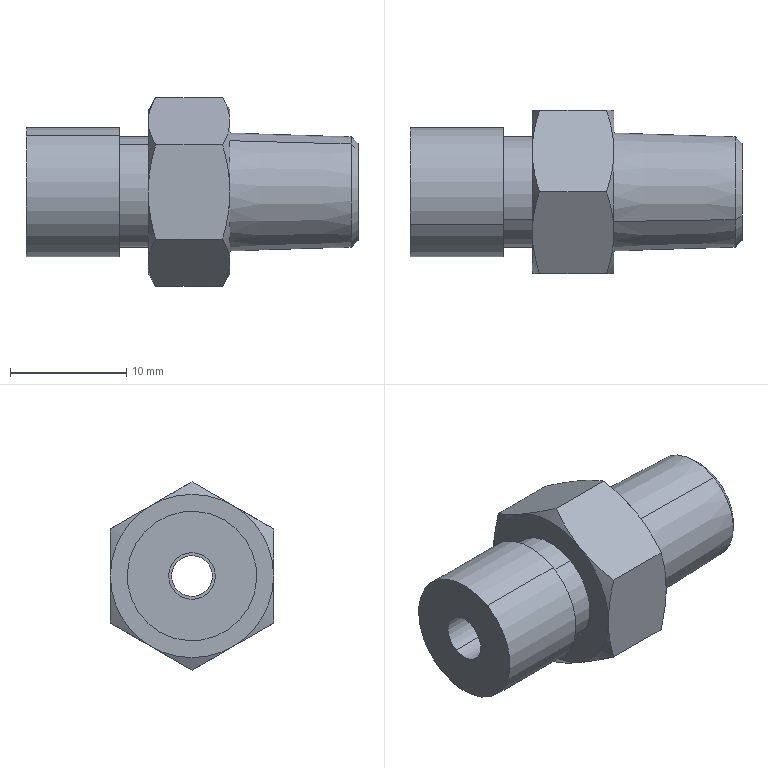Part | STEP file | SKTGK4-1-Part-1-1 | 1 solid | 36 faces | box 28.5 x 14 x 16.166 mm | volume 2666 mm3 | cone 16 | plane 12 | cylinder 8 | commonest cylinder face diameters 3.5 x2 4 x2 9.5 x2 11.112 x2
STEP:
#1=CARTESIAN_POINT('',(15.3,4.625,12.197));
#2=VERTEX_POINT('',#1);
#3=CARTESIAN_POINT('',(15.3,9.375,3.969));
#4=VERTEX_POINT('',#3);
#5=CARTESIAN_POINT('',(15.3,7.,8.083));
#6=DIRECTION('',(1.,0.,0.));
#7=DIRECTION('',(0.,-0.5,0.866));
#8=AXIS2_PLACEMENT_3D('',#5,#6,#7);
#9=CIRCLE('',#8,4.75);
#10=EDGE_CURVE('',#2,#4,#9,.T.);
#11=ORIENTED_EDGE('',*,*,#10,.T.);
#12=CARTESIAN_POINT('',(17.8,9.375,3.969));
#13=VERTEX_POINT('',#12);
#14=CARTESIAN_POINT('',(35.8,9.375,3.969));
#15=DIRECTION('',(1.,0.,0.));
#16=VECTOR('',#15,1000.);
#17=LINE('',#14,#16);
#18=EDGE_CURVE('',#4,#13,#17,.T.);
#19=ORIENTED_EDGE('',*,*,#18,.T.);
#20=CARTESIAN_POINT('',(17.8,4.625,12.197));
#21=VERTEX_POINT('',#20);
#22=CARTESIAN_POINT('',(17.8,7.,8.083));
#23=DIRECTION('',(1.,0.,0.));
#24=DIRECTION('',(0.,-0.5,0.866));
#25=AXIS2_PLACEMENT_3D('',#22,#23,#24);
#26=CIRCLE('',#25,4.75);
#27=EDGE_CURVE('',#21,#13,#26,.T.);
#28=ORIENTED_EDGE('',*,*,#27,.F.);
#29=CARTESIAN_POINT('',(35.8,4.625,12.197));
#30=DIRECTION('',(1.,0.,0.));
#31=VECTOR('',#30,1000.);
#32=LINE('',#29,#31);
#33=EDGE_CURVE('',#2,#21,#32,.T.);
#34=ORIENTED_EDGE('',*,*,#33,.F.);
#35=EDGE_LOOP('',(#11,#19,#28,#34));
#36=FACE_OUTER_BOUND('',#35,.T.);
#37=CARTESIAN_POINT('',(35.8,7.,8.083));
#38=DIRECTION('',(1.,0.,0.));
#39=DIRECTION('',(0.,-0.5,0.866));
#40=AXIS2_PLACEMENT_3D('',#37,#38,#39);
#41=CYLINDRICAL_SURFACE('',#40,4.75);
#42=ADVANCED_FACE('',(#36),#41,.T.);
#43=CARTESIAN_POINT('',(35.2,4.621,12.203));
#44=VERTEX_POINT('',#43);
#45=CARTESIAN_POINT('',(35.2,9.379,3.962));
#46=VERTEX_POINT('',#45);
#47=CARTESIAN_POINT('',(35.2,7.,8.083));
#48=DIRECTION('',(1.,0.,0.));
#49=DIRECTION('',(0.,-0.5,0.866));
#50=AXIS2_PLACEMENT_3D('',#47,#48,#49);
#51=CIRCLE('',#50,4.758);
#52=EDGE_CURVE('',#44,#46,#51,.T.);
#53=ORIENTED_EDGE('',*,*,#52,.F.);
#54=CARTESIAN_POINT('',(24.8,4.459,12.485));
#55=VERTEX_POINT('',#54);
#56=CARTESIAN_POINT('',(35.2,4.621,12.203));
#57=DIRECTION('',(-0.9995,-0.0156,0.02702));
#58=VECTOR('',#57,1000.);
#59=LINE('',#56,#58);
#60=EDGE_CURVE('',#44,#55,#59,.T.);
#61=ORIENTED_EDGE('',*,*,#60,.T.);
#62=CARTESIAN_POINT('',(24.8,9.541,3.681));
#63=VERTEX_POINT('',#62);
#64=CARTESIAN_POINT('',(24.8,7.,8.083));
#65=DIRECTION('',(1.,0.,0.));
#66=DIRECTION('',(0.,-0.5,0.866));
#67=AXIS2_PLACEMENT_3D('',#64,#65,#66);
#68=CIRCLE('',#67,5.083);
#69=EDGE_CURVE('',#55,#63,#68,.T.);
#70=ORIENTED_EDGE('',*,*,#69,.T.);
#71=CARTESIAN_POINT('',(35.2,9.379,3.962));
#72=DIRECTION('',(-0.9995,0.0156,-0.02702));
#73=VECTOR('',#72,1000.);
#74=LINE('',#71,#73);
#75=EDGE_CURVE('',#46,#63,#74,.T.);
#76=ORIENTED_EDGE('',*,*,#75,.F.);
#77=EDGE_LOOP('',(#53,#61,#70,#76));
#78=FACE_OUTER_BOUND('',#77,.T.);
#79=CARTESIAN_POINT('',(35.2,7.,8.083));
#80=DIRECTION('',(-1.,0.,0.));
#81=DIRECTION('',(0.,0.5,-0.866));
#82=AXIS2_PLACEMENT_3D('',#79,#80,#81);
#83=CONICAL_SURFACE('',#82,4.758,0.03121);
#84=ADVANCED_FACE('',(#78),#83,.T.);
#85=CARTESIAN_POINT('',(35.8,4.921,11.684));
#86=VERTEX_POINT('',#85);
#87=CARTESIAN_POINT('',(35.8,9.079,4.482));
#88=VERTEX_POINT('',#87);
#89=CARTESIAN_POINT('',(35.8,7.,8.083));
#90=DIRECTION('',(1.,0.,0.));
#91=DIRECTION('',(0.,-0.5,0.866));
#92=AXIS2_PLACEMENT_3D('',#89,#90,#91);
#93=CIRCLE('',#92,4.158);
#94=EDGE_CURVE('',#86,#88,#93,.T.);
#95=ORIENTED_EDGE('',*,*,#94,.F.);
#96=CARTESIAN_POINT('',(35.8,4.921,11.684));
#97=DIRECTION('',(-0.7071,-0.3536,0.6124));
#98=VECTOR('',#97,1000.);
#99=LINE('',#96,#98);
#100=EDGE_CURVE('',#86,#44,#99,.T.);
#101=ORIENTED_EDGE('',*,*,#100,.T.);
#102=ORIENTED_EDGE('',*,*,#52,.T.);
#103=CARTESIAN_POINT('',(35.8,9.079,4.482));
#104=DIRECTION('',(-0.7071,0.3536,-0.6124));
#105=VECTOR('',#104,1000.);
#106=LINE('',#103,#105);
#107=EDGE_CURVE('',#88,#46,#106,.T.);
#108=ORIENTED_EDGE('',*,*,#107,.F.);
#109=EDGE_LOOP('',(#95,#101,#102,#108));
#110=FACE_OUTER_BOUND('',#109,.T.);
#111=CARTESIAN_POINT('',(35.8,7.,8.083));
#112=DIRECTION('',(-1.,0.,0.));
#113=DIRECTION('',(0.,0.5,-0.866));
#114=AXIS2_PLACEMENT_3D('',#111,#112,#113);
#115=CONICAL_SURFACE('',#114,4.158,0.7854);
#116=ADVANCED_FACE('',(#110),#115,.T.);
#117=CARTESIAN_POINT('',(15.3,7.875,6.567));
#118=VERTEX_POINT('',#117);
#119=CARTESIAN_POINT('',(15.3,6.125,9.598));
#120=VERTEX_POINT('',#119);
#121=CARTESIAN_POINT('',(15.3,7.,8.083));
#122=DIRECTION('',(1.,0.,0.));
#123=DIRECTION('',(0.,-0.5,0.866));
#124=AXIS2_PLACEMENT_3D('',#121,#122,#123);
#125=CIRCLE('',#124,1.75);
#126=EDGE_CURVE('',#118,#120,#125,.T.);
#127=ORIENTED_EDGE('',*,*,#126,.F.);
#128=CARTESIAN_POINT('',(35.8,7.875,6.567));
#129=VERTEX_POINT('',#128);
#130=CARTESIAN_POINT('',(35.8,7.875,6.567));
#131=DIRECTION('',(1.,0.,0.));
#132=VECTOR('',#131,1000.);
#133=LINE('',#130,#132);
#134=EDGE_CURVE('',#118,#129,#133,.T.);
#135=ORIENTED_EDGE('',*,*,#134,.T.);
#136=CARTESIAN_POINT('',(35.8,6.125,9.598));
#137=VERTEX_POINT('',#136);
#138=CARTESIAN_POINT('',(35.8,7.,8.083));
#139=DIRECTION('',(1.,0.,0.));
#140=DIRECTION('',(0.,-0.5,0.866));
#141=AXIS2_PLACEMENT_3D('',#138,#139,#140);
#142=CIRCLE('',#141,1.75);
#143=EDGE_CURVE('',#129,#137,#142,.T.);
#144=ORIENTED_EDGE('',*,*,#143,.T.);
#145=CARTESIAN_POINT('',(35.8,6.125,9.598));
#146=DIRECTION('',(1.,0.,0.));
#147=VECTOR('',#146,1000.);
#148=LINE('',#145,#147);
#149=EDGE_CURVE('',#120,#137,#148,.T.);
#150=ORIENTED_EDGE('',*,*,#149,.F.);
#151=EDGE_LOOP('',(#127,#135,#144,#150));
#152=FACE_OUTER_BOUND('',#151,.T.);
#153=CARTESIAN_POINT('',(35.8,7.,8.083));
#154=DIRECTION('',(1.,0.,0.));
#155=DIRECTION('',(0.,-0.5,0.866));
#156=AXIS2_PLACEMENT_3D('',#153,#154,#155);
#157=CYLINDRICAL_SURFACE('',#156,1.75);
#158=ADVANCED_FACE('',(#152),#157,.F.);
#159=CARTESIAN_POINT('',(7.3,8.,6.351));
#160=VERTEX_POINT('',#159);
#161=CARTESIAN_POINT('',(7.3,6.,9.815));
#162=VERTEX_POINT('',#161);
#163=CARTESIAN_POINT('',(7.3,7.,8.083));
#164=DIRECTION('',(1.,0.,0.));
#165=DIRECTION('',(0.,-0.5,0.866));
#166=AXIS2_PLACEMENT_3D('',#163,#164,#165);
#167=CIRCLE('',#166,2.);
#168=EDGE_CURVE('',#160,#162,#167,.T.);
#169=ORIENTED_EDGE('',*,*,#168,.F.);
#170=CARTESIAN_POINT('',(15.3,8.,6.351));
#171=VERTEX_POINT('',#170);
#172=CARTESIAN_POINT('',(35.8,8.,6.351));
#173=DIRECTION('',(1.,0.,0.));
#174=VECTOR('',#173,1000.);
#175=LINE('',#172,#174);
#176=EDGE_CURVE('',#160,#171,#175,.T.);
#177=ORIENTED_EDGE('',*,*,#176,.T.);
#178=CARTESIAN_POINT('',(15.3,6.,9.815));
#179=VERTEX_POINT('',#178);
#180=CARTESIAN_POINT('',(15.3,7.,8.083));
#181=DIRECTION('',(1.,0.,0.));
#182=DIRECTION('',(0.,-0.5,0.866));
#183=AXIS2_PLACEMENT_3D('',#180,#181,#182);
#184=CIRCLE('',#183,2.);
#185=EDGE_CURVE('',#171,#179,#184,.T.);
#186=ORIENTED_EDGE('',*,*,#185,.T.);
#187=CARTESIAN_POINT('',(35.8,6.,9.815));
#188=DIRECTION('',(1.,0.,0.));
#189=VECTOR('',#188,1000.);
#190=LINE('',#187,#189);
#191=EDGE_CURVE('',#162,#179,#190,.T.);
#192=ORIENTED_EDGE('',*,*,#191,.F.);
#193=EDGE_LOOP('',(#169,#177,#186,#192));
#194=FACE_OUTER_BOUND('',#193,.T.);
#195=CARTESIAN_POINT('',(35.8,7.,8.083));
#196=DIRECTION('',(1.,0.,0.));
#197=DIRECTION('',(0.,-0.5,0.866));
#198=AXIS2_PLACEMENT_3D('',#195,#196,#197);
#199=CYLINDRICAL_SURFACE('',#198,2.);
#200=ADVANCED_FACE('',(#194),#199,.F.);
#201=CARTESIAN_POINT('',(7.3,4.222,12.895));
#202=VERTEX_POINT('',#201);
#203=CARTESIAN_POINT('',(7.3,9.778,3.271));
#204=VERTEX_POINT('',#203);
#205=CARTESIAN_POINT('',(7.3,7.,8.083));
#206=DIRECTION('',(1.,0.,0.));
#207=DIRECTION('',(0.,-0.5,0.866));
#208=AXIS2_PLACEMENT_3D('',#205,#206,#207);
#209=CIRCLE('',#208,5.556);
#210=EDGE_CURVE('',#202,#204,#209,.T.);
#211=ORIENTED_EDGE('',*,*,#210,.T.);
#212=CARTESIAN_POINT('',(15.3,9.778,3.271));
#213=VERTEX_POINT('',#212);
#214=CARTESIAN_POINT('',(35.8,9.778,3.271));
#215=DIRECTION('',(1.,0.,0.));
#216=VECTOR('',#215,1000.);
#217=LINE('',#214,#216);
#218=EDGE_CURVE('',#204,#213,#217,.T.);
#219=ORIENTED_EDGE('',*,*,#218,.T.);
#220=CARTESIAN_POINT('',(15.3,4.222,12.895));
#221=VERTEX_POINT('',#220);
#222=CARTESIAN_POINT('',(15.3,7.,8.083));
#223=DIRECTION('',(1.,0.,0.));
#224=DIRECTION('',(0.,-0.5,0.866));
#225=AXIS2_PLACEMENT_3D('',#222,#223,#224);
#226=CIRCLE('',#225,5.556);
#227=EDGE_CURVE('',#221,#213,#226,.T.);
#228=ORIENTED_EDGE('',*,*,#227,.F.);
#229=CARTESIAN_POINT('',(35.8,4.222,12.895));
#230=DIRECTION('',(1.,0.,0.));
#231=VECTOR('',#230,1000.);
#232=LINE('',#229,#231);
#233=EDGE_CURVE('',#202,#221,#232,.T.);
#234=ORIENTED_EDGE('',*,*,#233,.F.);
#235=EDGE_LOOP('',(#211,#219,#228,#234));
#236=FACE_OUTER_BOUND('',#235,.T.);
#237=CARTESIAN_POINT('',(35.8,7.,8.083));
#238=DIRECTION('',(1.,0.,0.));
#239=DIRECTION('',(0.,-0.5,0.866));
#240=AXIS2_PLACEMENT_3D('',#237,#238,#239);
#241=CYLINDRICAL_SURFACE('',#240,5.556);
#242=ADVANCED_FACE('',(#236),#241,.T.);
#243=CARTESIAN_POINT('',(24.8,3.5,14.145));
#244=VERTEX_POINT('',#243);
#245=CARTESIAN_POINT('',(24.175,0.,12.124));
#246=VERTEX_POINT('',#245);
#247=CARTESIAN_POINT('',(24.8,3.5,14.145));
#248=CARTESIAN_POINT('',(24.8,2.302,13.454));
#249=CARTESIAN_POINT('',(24.555,1.141,12.783));
#250=CARTESIAN_POINT('',(24.175,0.,12.124));
#251=B_SPLINE_CURVE_WITH_KNOTS('',3,(#247,#248,#249,#250),.UNSPECIFIED.,.F.,.F.,(4,4),(0.0137,0.01782),.UNSPECIFIED.);
#252=EDGE_CURVE('',#244,#246,#251,.T.);
#253=ORIENTED_EDGE('',*,*,#252,.T.);
#254=CARTESIAN_POINT('',(24.8,0.,8.083));
#255=VERTEX_POINT('',#254);
#256=CARTESIAN_POINT('',(24.175,0.,12.124));
#257=CARTESIAN_POINT('',(24.366,0.,11.463));
#258=CARTESIAN_POINT('',(24.523,0.,10.797));
#259=CARTESIAN_POINT('',(24.74,0.,9.451));
#260=CARTESIAN_POINT('',(24.8,0.,8.771));
#261=CARTESIAN_POINT('',(24.8,0.,8.083));
#262=B_SPLINE_CURVE_WITH_KNOTS('',3,(#256,#257,#258,#259,#260,#261),.UNSPECIFIED.,.F.,.F.,(4,2,4),(0.000000238,0.002045,0.00409),.UNSPECIFIED.);
#263=EDGE_CURVE('',#246,#255,#262,.T.);
#264=ORIENTED_EDGE('',*,*,#263,.T.);
#265=CARTESIAN_POINT('',(24.8,7.,8.083));
#266=DIRECTION('',(1.,0.,0.));
#267=DIRECTION('',(0.,-0.5,0.866));
#268=AXIS2_PLACEMENT_3D('',#265,#266,#267);
#269=CIRCLE('',#268,7.);
#270=EDGE_CURVE('',#244,#255,#269,.T.);
#271=ORIENTED_EDGE('',*,*,#270,.F.);
#272=EDGE_LOOP('',(#253,#264,#271));
#273=FACE_OUTER_BOUND('',#272,.T.);
#274=CARTESIAN_POINT('',(24.8,7.,8.083));
#275=DIRECTION('',(-1.,0.,0.));
#276=DIRECTION('',(0.,0.5,-0.866));
#277=AXIS2_PLACEMENT_3D('',#274,#275,#276);
#278=CONICAL_SURFACE('',#277,7.,1.047);
#279=ADVANCED_FACE('',(#273),#278,.T.);
#280=CARTESIAN_POINT('',(24.8,3.5,2.021));
#281=VERTEX_POINT('',#280);
#282=CARTESIAN_POINT('',(24.8,7.,8.083));
#283=DIRECTION('',(1.,0.,0.));
#284=DIRECTION('',(0.,-0.5,0.866));
#285=AXIS2_PLACEMENT_3D('',#282,#283,#284);
#286=CIRCLE('',#285,7.);
#287=EDGE_CURVE('',#255,#281,#286,.T.);
#288=ORIENTED_EDGE('',*,*,#287,.F.);
#289=CARTESIAN_POINT('',(24.175,0.,4.041));
#290=VERTEX_POINT('',#289);
#291=CARTESIAN_POINT('',(24.8,0.,8.083));
#292=CARTESIAN_POINT('',(24.8,0.,7.74));
#293=CARTESIAN_POINT('',(24.785,0.,7.395));
#294=CARTESIAN_POINT('',(24.728,0.,6.714));
#295=CARTESIAN_POINT('',(24.686,0.,6.375));
#296=CARTESIAN_POINT('',(24.522,0.,5.366));
#297=CARTESIAN_POINT('',(24.365,0.,4.701));
#298=CARTESIAN_POINT('',(24.175,0.,4.041));
#299=B_SPLINE_CURVE_WITH_KNOTS('',3,(#291,#292,#293,#294,#295,#296,#297,#298),.UNSPECIFIED.,.F.,.F.,(4,2,2,4),(0.00409,0.005108,0.006127,0.008164),.UNSPECIFIED.);
#300=EDGE_CURVE('',#255,#290,#299,.T.);
#301=ORIENTED_EDGE('',*,*,#300,.T.);
#302=CARTESIAN_POINT('',(24.175,0.,4.041));
#303=CARTESIAN_POINT('',(24.366,0.5726,3.711));
#304=CARTESIAN_POINT('',(24.523,1.149,3.378));
#305=CARTESIAN_POINT('',(24.74,2.315,2.705));
#306=CARTESIAN_POINT('',(24.8,2.904,2.365));
#307=CARTESIAN_POINT('',(24.8,3.5,2.021));
#308=B_SPLINE_CURVE_WITH_KNOTS('',3,(#302,#303,#304,#305,#306,#307),.UNSPECIFIED.,.F.,.F.,(4,2,4),(0.000000238,0.002045,0.00409),.UNSPECIFIED.);
#309=EDGE_CURVE('',#290,#281,#308,.T.);
#310=ORIENTED_EDGE('',*,*,#309,.T.);
#311=EDGE_LOOP('',(#288,#301,#310));
#312=FACE_OUTER_BOUND('',#311,.T.);
#313=CARTESIAN_POINT('',(24.8,7.,8.083));
#314=DIRECTION('',(-1.,0.,0.));
#315=DIRECTION('',(0.,0.5,-0.866));
#316=AXIS2_PLACEMENT_3D('',#313,#314,#315);
#317=CONICAL_SURFACE('',#316,7.,1.047);
#318=ADVANCED_FACE('',(#312),#317,.T.);
#319=CARTESIAN_POINT('',(24.8,10.5,2.021));
#320=VERTEX_POINT('',#319);
#321=CARTESIAN_POINT('',(24.8,7.,8.083));
#322=DIRECTION('',(1.,0.,0.));
#323=DIRECTION('',(0.,-0.5,0.866));
#324=AXIS2_PLACEMENT_3D('',#321,#322,#323);
#325=CIRCLE('',#324,7.);
#326=EDGE_CURVE('',#281,#320,#325,.T.);
#327=ORIENTED_EDGE('',*,*,#326,.F.);
#328=CARTESIAN_POINT('',(24.175,7.,0.));
#329=VERTEX_POINT('',#328);
#330=CARTESIAN_POINT('',(24.8,3.5,2.021));
#331=CARTESIAN_POINT('',(24.8,3.797,1.849));
#332=CARTESIAN_POINT('',(24.785,4.095,1.677));
#333=CARTESIAN_POINT('',(24.728,4.686,1.336));
#334=CARTESIAN_POINT('',(24.686,4.979,1.167));
#335=CARTESIAN_POINT('',(24.522,5.853,0.6622));
#336=CARTESIAN_POINT('',(24.365,6.429,0.3297));
#337=CARTESIAN_POINT('',(24.175,7.,0.));
#338=B_SPLINE_CURVE_WITH_KNOTS('',3,(#330,#331,#332,#333,#334,#335,#336,#337),.UNSPECIFIED.,.F.,.F.,(4,2,2,4),(0.00409,0.005108,0.006127,0.008164),.UNSPECIFIED.);
#339=EDGE_CURVE('',#281,#329,#338,.T.);
#340=ORIENTED_EDGE('',*,*,#339,.T.);
#341=CARTESIAN_POINT('',(24.175,7.,0.));
#342=CARTESIAN_POINT('',(24.364,7.569,0.3283));
#343=CARTESIAN_POINT('',(24.521,8.143,0.6599));
#344=CARTESIAN_POINT('',(24.685,9.017,1.164));
#345=CARTESIAN_POINT('',(24.728,9.31,1.334));
#346=CARTESIAN_POINT('',(24.785,9.902,1.675));
#347=CARTESIAN_POINT('',(24.8,10.201,1.848));
#348=CARTESIAN_POINT('',(24.8,10.5,2.021));
#349=B_SPLINE_CURVE_WITH_KNOTS('',3,(#341,#342,#343,#344,#345,#346,#347,#348),.UNSPECIFIED.,.F.,.F.,(4,2,2,4),(0.009591,0.01165,0.01267,0.0137),.UNSPECIFIED.);
#350=EDGE_CURVE('',#329,#320,#349,.T.);
#351=ORIENTED_EDGE('',*,*,#350,.T.);
#352=EDGE_LOOP('',(#327,#340,#351));
#353=FACE_OUTER_BOUND('',#352,.T.);
#354=CARTESIAN_POINT('',(24.8,7.,8.083));
#355=DIRECTION('',(-1.,0.,0.));
#356=DIRECTION('',(0.,0.5,-0.866));
#357=AXIS2_PLACEMENT_3D('',#354,#355,#356);
#358=CONICAL_SURFACE('',#357,7.,1.047);
#359=ADVANCED_FACE('',(#353),#358,.T.);
#360=CARTESIAN_POINT('',(24.8,10.5,14.145));
#361=VERTEX_POINT('',#360);
#362=CARTESIAN_POINT('',(24.175,7.,16.166));
#363=VERTEX_POINT('',#362);
#364=CARTESIAN_POINT('',(24.8,10.5,14.145));
#365=CARTESIAN_POINT('',(24.8,10.203,14.317));
#366=CARTESIAN_POINT('',(24.785,9.905,14.489));
#367=CARTESIAN_POINT('',(24.728,9.314,14.83));
#368=CARTESIAN_POINT('',(24.686,9.021,14.999));
#369=CARTESIAN_POINT('',(24.522,8.147,15.504));
#370=CARTESIAN_POINT('',(24.365,7.571,15.836));
#371=CARTESIAN_POINT('',(24.175,7.,16.166));
#372=B_SPLINE_CURVE_WITH_KNOTS('',3,(#364,#365,#366,#367,#368,#369,#370,#371),.UNSPECIFIED.,.F.,.F.,(4,2,2,4),(0.00409,0.005108,0.006127,0.008164),.UNSPECIFIED.);
#373=EDGE_CURVE('',#361,#363,#372,.T.);
#374=ORIENTED_EDGE('',*,*,#373,.T.);
#375=CARTESIAN_POINT('',(24.175,7.,16.166));
#376=CARTESIAN_POINT('',(24.364,6.431,15.837));
#377=CARTESIAN_POINT('',(24.521,5.857,15.506));
#378=CARTESIAN_POINT('',(24.685,4.983,15.001));
#379=CARTESIAN_POINT('',(24.728,4.69,14.832));
#380=CARTESIAN_POINT('',(24.785,4.098,14.49));
#381=CARTESIAN_POINT('',(24.8,3.799,14.318));
#382=CARTESIAN_POINT('',(24.8,3.5,14.145));
#383=B_SPLINE_CURVE_WITH_KNOTS('',3,(#375,#376,#377,#378,#379,#380,#381,#382),.UNSPECIFIED.,.F.,.F.,(4,2,2,4),(0.009591,0.01165,0.01267,0.0137),.UNSPECIFIED.);
#384=EDGE_CURVE('',#363,#244,#383,.T.);
#385=ORIENTED_EDGE('',*,*,#384,.T.);
#386=CARTESIAN_POINT('',(24.8,7.,8.083));
#387=DIRECTION('',(1.,0.,0.));
#388=DIRECTION('',(0.,-0.5,0.866));
#389=AXIS2_PLACEMENT_3D('',#386,#387,#388);
#390=CIRCLE('',#389,7.);
#391=EDGE_CURVE('',#361,#244,#390,.T.);
#392=ORIENTED_EDGE('',*,*,#391,.F.);
#393=EDGE_LOOP('',(#374,#385,#392));
#394=FACE_OUTER_BOUND('',#393,.T.);
#395=CARTESIAN_POINT('',(24.8,7.,8.083));
#396=DIRECTION('',(-1.,0.,0.));
#397=DIRECTION('',(0.,0.5,-0.866));
#398=AXIS2_PLACEMENT_3D('',#395,#396,#397);
#399=CONICAL_SURFACE('',#398,7.,1.047);
#400=ADVANCED_FACE('',(#394),#399,.T.);
#401=CARTESIAN_POINT('',(24.8,14.,8.083));
#402=VERTEX_POINT('',#401);
#403=CARTESIAN_POINT('',(24.8,7.,8.083));
#404=DIRECTION('',(1.,0.,0.));
#405=DIRECTION('',(0.,-0.5,0.866));
#406=AXIS2_PLACEMENT_3D('',#403,#404,#405);
#407=CIRCLE('',#406,7.);
#408=EDGE_CURVE('',#320,#402,#407,.T.);
#409=ORIENTED_EDGE('',*,*,#408,.F.);
#410=CARTESIAN_POINT('',(24.175,14.,4.041));
#411=VERTEX_POINT('',#410);
#412=CARTESIAN_POINT('',(24.8,10.5,2.021));
#413=CARTESIAN_POINT('',(24.8,11.698,2.712));
#414=CARTESIAN_POINT('',(24.555,12.859,3.383));
#415=CARTESIAN_POINT('',(24.175,14.,4.041));
#416=B_SPLINE_CURVE_WITH_KNOTS('',3,(#412,#413,#414,#415),.UNSPECIFIED.,.F.,.F.,(4,4),(0.0137,0.01782),.UNSPECIFIED.);
#417=EDGE_CURVE('',#320,#411,#416,.T.);
#418=ORIENTED_EDGE('',*,*,#417,.T.);
#419=CARTESIAN_POINT('',(24.175,14.,4.041));
#420=CARTESIAN_POINT('',(24.366,14.,4.703));
#421=CARTESIAN_POINT('',(24.523,14.,5.369));
#422=CARTESIAN_POINT('',(24.74,14.,6.714));
#423=CARTESIAN_POINT('',(24.8,14.,7.394));
#424=CARTESIAN_POINT('',(24.8,14.,8.083));
#425=B_SPLINE_CURVE_WITH_KNOTS('',3,(#419,#420,#421,#422,#423,#424),.UNSPECIFIED.,.F.,.F.,(4,2,4),(0.000000238,0.002045,0.00409),.UNSPECIFIED.);
#426=EDGE_CURVE('',#411,#402,#425,.T.);
#427=ORIENTED_EDGE('',*,*,#426,.T.);
#428=EDGE_LOOP('',(#409,#418,#427));
#429=FACE_OUTER_BOUND('',#428,.T.);
#430=CARTESIAN_POINT('',(24.8,7.,8.083));
#431=DIRECTION('',(-1.,0.,0.));
#432=DIRECTION('',(0.,0.5,-0.866));
#433=AXIS2_PLACEMENT_3D('',#430,#431,#432);
#434=CONICAL_SURFACE('',#433,7.,1.047);
#435=ADVANCED_FACE('',(#429),#434,.T.);
#436=CARTESIAN_POINT('',(24.175,14.,12.124));
#437=VERTEX_POINT('',#436);
#438=CARTESIAN_POINT('',(24.8,14.,8.083));
#439=CARTESIAN_POINT('',(24.8,14.,8.426));
#440=CARTESIAN_POINT('',(24.785,14.,8.77));
#441=CARTESIAN_POINT('',(24.728,14.,9.452));
#442=CARTESIAN_POINT('',(24.686,14.,9.79));
#443=CARTESIAN_POINT('',(24.522,14.,10.8));
#444=CARTESIAN_POINT('',(24.365,14.,11.465));
#445=CARTESIAN_POINT('',(24.175,14.,12.124));
#446=B_SPLINE_CURVE_WITH_KNOTS('',3,(#438,#439,#440,#441,#442,#443,#444,#445),.UNSPECIFIED.,.F.,.F.,(4,2,2,4),(0.00409,0.005108,0.006127,0.008164),.UNSPECIFIED.);
#447=EDGE_CURVE('',#402,#437,#446,.T.);
#448=ORIENTED_EDGE('',*,*,#447,.T.);
#449=CARTESIAN_POINT('',(24.175,14.,12.124));
#450=CARTESIAN_POINT('',(24.366,13.427,12.455));
#451=CARTESIAN_POINT('',(24.523,12.851,12.788));
#452=CARTESIAN_POINT('',(24.74,11.685,13.461));
#453=CARTESIAN_POINT('',(24.8,11.096,13.801));
#454=CARTESIAN_POINT('',(24.8,10.5,14.145));
#455=B_SPLINE_CURVE_WITH_KNOTS('',3,(#449,#450,#451,#452,#453,#454),.UNSPECIFIED.,.F.,.F.,(4,2,4),(0.000000238,0.002045,0.00409),.UNSPECIFIED.);
#456=EDGE_CURVE('',#437,#361,#455,.T.);
#457=ORIENTED_EDGE('',*,*,#456,.T.);
#458=CARTESIAN_POINT('',(24.8,7.,8.083));
#459=DIRECTION('',(1.,0.,0.));
#460=DIRECTION('',(0.,-0.5,0.866));
#461=AXIS2_PLACEMENT_3D('',#458,#459,#460);
#462=CIRCLE('',#461,7.);
#463=EDGE_CURVE('',#402,#361,#462,.T.);
#464=ORIENTED_EDGE('',*,*,#463,.F.);
#465=EDGE_LOOP('',(#448,#457,#464));
#466=FACE_OUTER_BOUND('',#465,.T.);
#467=CARTESIAN_POINT('',(24.8,7.,8.083));
#468=DIRECTION('',(-1.,0.,0.));
#469=DIRECTION('',(0.,0.5,-0.866));
#470=AXIS2_PLACEMENT_3D('',#467,#468,#469);
#471=CONICAL_SURFACE('',#470,7.,1.047);
#472=ADVANCED_FACE('',(#466),#471,.T.);
#473=CARTESIAN_POINT('',(17.8,14.,8.083));
#474=VERTEX_POINT('',#473);
#475=CARTESIAN_POINT('',(18.425,14.,4.041));
#476=VERTEX_POINT('',#475);
#477=CARTESIAN_POINT('',(17.8,14.,8.083));
#478=CARTESIAN_POINT('',(17.8,14.,7.74));
#479=CARTESIAN_POINT('',(17.815,14.,7.395));
#480=CARTESIAN_POINT('',(17.872,14.,6.714));
#481=CARTESIAN_POINT('',(17.914,14.,6.375));
#482=CARTESIAN_POINT('',(18.078,14.,5.366));
#483=CARTESIAN_POINT('',(18.235,14.,4.701));
#484=CARTESIAN_POINT('',(18.425,14.,4.041));
#485=B_SPLINE_CURVE_WITH_KNOTS('',3,(#477,#478,#479,#480,#481,#482,#483,#484),.UNSPECIFIED.,.F.,.F.,(4,2,2,4),(0.00409,0.005108,0.006127,0.008164),.UNSPECIFIED.);
#486=EDGE_CURVE('',#474,#476,#485,.T.);
#487=ORIENTED_EDGE('',*,*,#486,.T.);
#488=CARTESIAN_POINT('',(17.8,10.5,2.021));
#489=VERTEX_POINT('',#488);
#490=CARTESIAN_POINT('',(18.425,14.,4.041));
#491=CARTESIAN_POINT('',(18.236,13.431,3.713));
#492=CARTESIAN_POINT('',(18.079,12.857,3.382));
#493=CARTESIAN_POINT('',(17.915,11.983,2.877));
#494=CARTESIAN_POINT('',(17.872,11.69,2.708));
#495=CARTESIAN_POINT('',(17.815,11.098,2.366));
#496=CARTESIAN_POINT('',(17.8,10.799,2.193));
#497=CARTESIAN_POINT('',(17.8,10.5,2.021));
#498=B_SPLINE_CURVE_WITH_KNOTS('',3,(#490,#491,#492,#493,#494,#495,#496,#497),.UNSPECIFIED.,.F.,.F.,(4,2,2,4),(0.009591,0.01165,0.01267,0.0137),.UNSPECIFIED.);
#499=EDGE_CURVE('',#476,#489,#498,.T.);
#500=ORIENTED_EDGE('',*,*,#499,.T.);
#501=CARTESIAN_POINT('',(17.8,7.,8.083));
#502=DIRECTION('',(1.,0.,0.));
#503=DIRECTION('',(0.,-0.5,0.866));
#504=AXIS2_PLACEMENT_3D('',#501,#502,#503);
#505=CIRCLE('',#504,7.);
#506=EDGE_CURVE('',#489,#474,#505,.T.);
#507=ORIENTED_EDGE('',*,*,#506,.T.);
#508=EDGE_LOOP('',(#487,#500,#507));
#509=FACE_OUTER_BOUND('',#508,.T.);
#510=CARTESIAN_POINT('',(21.3,7.,8.083));
#511=DIRECTION('',(1.,0.,0.));
#512=DIRECTION('',(0.,-0.5,0.866));
#513=AXIS2_PLACEMENT_3D('',#510,#511,#512);
#514=CONICAL_SURFACE('',#513,13.062,1.047);
#515=ADVANCED_FACE('',(#509),#514,.T.);
#516=CARTESIAN_POINT('',(17.8,3.5,2.021));
#517=VERTEX_POINT('',#516);
#518=CARTESIAN_POINT('',(17.8,7.,8.083));
#519=DIRECTION('',(1.,0.,0.));
#520=DIRECTION('',(0.,-0.5,0.866));
#521=AXIS2_PLACEMENT_3D('',#518,#519,#520);
#522=CIRCLE('',#521,7.);
#523=EDGE_CURVE('',#517,#489,#522,.T.);
#524=ORIENTED_EDGE('',*,*,#523,.T.);
#525=CARTESIAN_POINT('',(18.425,7.,0.));
#526=VERTEX_POINT('',#525);
#527=CARTESIAN_POINT('',(17.8,10.5,2.021));
#528=CARTESIAN_POINT('',(17.8,9.302,1.329));
#529=CARTESIAN_POINT('',(18.045,8.141,0.6588));
#530=CARTESIAN_POINT('',(18.425,7.,0.));
#531=B_SPLINE_CURVE_WITH_KNOTS('',3,(#527,#528,#529,#530),.UNSPECIFIED.,.F.,.F.,(4,4),(0.0137,0.01782),.UNSPECIFIED.);
#532=EDGE_CURVE('',#489,#526,#531,.T.);
#533=ORIENTED_EDGE('',*,*,#532,.T.);
#534=CARTESIAN_POINT('',(18.425,7.,0.));
#535=CARTESIAN_POINT('',(18.234,6.427,0.3306));
#536=CARTESIAN_POINT('',(18.077,5.851,0.6635));
#537=CARTESIAN_POINT('',(17.86,4.685,1.336));
#538=CARTESIAN_POINT('',(17.8,4.096,1.676));
#539=CARTESIAN_POINT('',(17.8,3.5,2.021));
#540=B_SPLINE_CURVE_WITH_KNOTS('',3,(#534,#535,#536,#537,#538,#539),.UNSPECIFIED.,.F.,.F.,(4,2,4),(0.000000238,0.002045,0.00409),.UNSPECIFIED.);
#541=EDGE_CURVE('',#526,#517,#540,.T.);
#542=ORIENTED_EDGE('',*,*,#541,.T.);
#543=EDGE_LOOP('',(#524,#533,#542));
#544=FACE_OUTER_BOUND('',#543,.T.);
#545=CARTESIAN_POINT('',(21.3,7.,8.083));
#546=DIRECTION('',(1.,0.,0.));
#547=DIRECTION('',(0.,-0.5,0.866));
#548=AXIS2_PLACEMENT_3D('',#545,#546,#547);
#549=CONICAL_SURFACE('',#548,13.062,1.047);
#550=ADVANCED_FACE('',(#544),#549,.T.);
#551=CARTESIAN_POINT('',(18.425,0.,4.041));
#552=VERTEX_POINT('',#551);
#553=CARTESIAN_POINT('',(17.8,0.,8.083));
#554=VERTEX_POINT('',#553);
#555=CARTESIAN_POINT('',(18.425,0.,4.041));
#556=CARTESIAN_POINT('',(18.234,0.,4.703));
#557=CARTESIAN_POINT('',(18.077,0.,5.369));
#558=CARTESIAN_POINT('',(17.86,0.,6.714));
#559=CARTESIAN_POINT('',(17.8,0.,7.394));
#560=CARTESIAN_POINT('',(17.8,0.,8.083));
#561=B_SPLINE_CURVE_WITH_KNOTS('',3,(#555,#556,#557,#558,#559,#560),.UNSPECIFIED.,.F.,.F.,(4,2,4),(0.000000238,0.002045,0.00409),.UNSPECIFIED.);
#562=EDGE_CURVE('',#552,#554,#561,.T.);
#563=ORIENTED_EDGE('',*,*,#562,.T.);
#564=CARTESIAN_POINT('',(17.8,7.,8.083));
#565=DIRECTION('',(1.,0.,0.));
#566=DIRECTION('',(0.,-0.5,0.866));
#567=AXIS2_PLACEMENT_3D('',#564,#565,#566);
#568=CIRCLE('',#567,7.);
#569=EDGE_CURVE('',#554,#517,#568,.T.);
#570=ORIENTED_EDGE('',*,*,#569,.T.);
#571=CARTESIAN_POINT('',(17.8,3.5,2.021));
#572=CARTESIAN_POINT('',(17.8,3.203,2.192));
#573=CARTESIAN_POINT('',(17.815,2.905,2.364));
#574=CARTESIAN_POINT('',(17.872,2.314,2.705));
#575=CARTESIAN_POINT('',(17.914,2.021,2.874));
#576=CARTESIAN_POINT('',(18.078,1.147,3.379));
#577=CARTESIAN_POINT('',(18.235,0.5711,3.712));
#578=CARTESIAN_POINT('',(18.425,0.,4.041));
#579=B_SPLINE_CURVE_WITH_KNOTS('',3,(#571,#572,#573,#574,#575,#576,#577,#578),.UNSPECIFIED.,.F.,.F.,(4,2,2,4),(0.00409,0.005108,0.006127,0.008164),.UNSPECIFIED.);
#580=EDGE_CURVE('',#517,#552,#579,.T.);
#581=ORIENTED_EDGE('',*,*,#580,.T.);
#582=EDGE_LOOP('',(#563,#570,#581));
#583=FACE_OUTER_BOUND('',#582,.T.);
#584=CARTESIAN_POINT('',(21.3,7.,8.083));
#585=DIRECTION('',(1.,0.,0.));
#586=DIRECTION('',(0.,-0.5,0.866));
#587=AXIS2_PLACEMENT_3D('',#584,#585,#586);
#588=CONICAL_SURFACE('',#587,13.062,1.047);
#589=ADVANCED_FACE('',(#583),#588,.T.);
#590=CARTESIAN_POINT('',(17.8,3.5,14.145));
#591=VERTEX_POINT('',#590);
#592=CARTESIAN_POINT('',(17.8,7.,8.083));
#593=DIRECTION('',(1.,0.,0.));
#594=DIRECTION('',(0.,-0.5,0.866));
#595=AXIS2_PLACEMENT_3D('',#592,#593,#594);
#596=CIRCLE('',#595,7.);
#597=EDGE_CURVE('',#591,#554,#596,.T.);
#598=ORIENTED_EDGE('',*,*,#597,.T.);
#599=CARTESIAN_POINT('',(18.425,0.,12.124));
#600=VERTEX_POINT('',#599);
#601=CARTESIAN_POINT('',(17.8,0.,8.083));
#602=CARTESIAN_POINT('',(17.8,0.,8.426));
#603=CARTESIAN_POINT('',(17.815,0.,8.77));
#604=CARTESIAN_POINT('',(17.872,0.,9.452));
#605=CARTESIAN_POINT('',(17.914,0.,9.79));
#606=CARTESIAN_POINT('',(18.078,0.,10.8));
#607=CARTESIAN_POINT('',(18.235,0.,11.465));
#608=CARTESIAN_POINT('',(18.425,0.,12.124));
#609=B_SPLINE_CURVE_WITH_KNOTS('',3,(#601,#602,#603,#604,#605,#606,#607,#608),.UNSPECIFIED.,.F.,.F.,(4,2,2,4),(0.00409,0.005108,0.006127,0.008164),.UNSPECIFIED.);
#610=EDGE_CURVE('',#554,#600,#609,.T.);
#611=ORIENTED_EDGE('',*,*,#610,.T.);
#612=CARTESIAN_POINT('',(18.425,0.,12.124));
#613=CARTESIAN_POINT('',(18.236,0.5687,12.453));
#614=CARTESIAN_POINT('',(18.079,1.143,12.784));
#615=CARTESIAN_POINT('',(17.915,2.017,13.289));
#616=CARTESIAN_POINT('',(17.872,2.31,13.458));
#617=CARTESIAN_POINT('',(17.815,2.902,13.8));
#618=CARTESIAN_POINT('',(17.8,3.201,13.973));
#619=CARTESIAN_POINT('',(17.8,3.5,14.145));
#620=B_SPLINE_CURVE_WITH_KNOTS('',3,(#612,#613,#614,#615,#616,#617,#618,#619),.UNSPECIFIED.,.F.,.F.,(4,2,2,4),(0.009591,0.01165,0.01267,0.0137),.UNSPECIFIED.);
#621=EDGE_CURVE('',#600,#591,#620,.T.);
#622=ORIENTED_EDGE('',*,*,#621,.T.);
#623=EDGE_LOOP('',(#598,#611,#622));
#624=FACE_OUTER_BOUND('',#623,.T.);
#625=CARTESIAN_POINT('',(21.3,7.,8.083));
#626=DIRECTION('',(1.,0.,0.));
#627=DIRECTION('',(0.,-0.5,0.866));
#628=AXIS2_PLACEMENT_3D('',#625,#626,#627);
#629=CONICAL_SURFACE('',#628,13.062,1.047);
#630=ADVANCED_FACE('',(#624),#629,.T.);
#631=CARTESIAN_POINT('',(17.8,10.5,14.145));
#632=VERTEX_POINT('',#631);
#633=CARTESIAN_POINT('',(17.8,7.,8.083));
#634=DIRECTION('',(1.,0.,0.));
#635=DIRECTION('',(0.,-0.5,0.866));
#636=AXIS2_PLACEMENT_3D('',#633,#634,#635);
#637=CIRCLE('',#636,7.);
#638=EDGE_CURVE('',#632,#591,#637,.T.);
#639=ORIENTED_EDGE('',*,*,#638,.T.);
#640=CARTESIAN_POINT('',(18.425,7.,16.166));
#641=VERTEX_POINT('',#640);
#642=CARTESIAN_POINT('',(17.8,3.5,14.145));
#643=CARTESIAN_POINT('',(17.8,4.698,14.837));
#644=CARTESIAN_POINT('',(18.045,5.859,15.507));
#645=CARTESIAN_POINT('',(18.425,7.,16.166));
#646=B_SPLINE_CURVE_WITH_KNOTS('',3,(#642,#643,#644,#645),.UNSPECIFIED.,.F.,.F.,(4,4),(0.0137,0.01782),.UNSPECIFIED.);
#647=EDGE_CURVE('',#591,#641,#646,.T.);
#648=ORIENTED_EDGE('',*,*,#647,.T.);
#649=CARTESIAN_POINT('',(18.425,7.,16.166));
#650=CARTESIAN_POINT('',(18.234,7.573,15.835));
#651=CARTESIAN_POINT('',(18.077,8.149,15.502));
#652=CARTESIAN_POINT('',(17.86,9.315,14.829));
#653=CARTESIAN_POINT('',(17.8,9.904,14.489));
#654=CARTESIAN_POINT('',(17.8,10.5,14.145));
#655=B_SPLINE_CURVE_WITH_KNOTS('',3,(#649,#650,#651,#652,#653,#654),.UNSPECIFIED.,.F.,.F.,(4,2,4),(0.000000238,0.002045,0.00409),.UNSPECIFIED.);
#656=EDGE_CURVE('',#641,#632,#655,.T.);
#657=ORIENTED_EDGE('',*,*,#656,.T.);
#658=EDGE_LOOP('',(#639,#648,#657));
#659=FACE_OUTER_BOUND('',#658,.T.);
#660=CARTESIAN_POINT('',(21.3,7.,8.083));
#661=DIRECTION('',(1.,0.,0.));
#662=DIRECTION('',(0.,-0.5,0.866));
#663=AXIS2_PLACEMENT_3D('',#660,#661,#662);
#664=CONICAL_SURFACE('',#663,13.062,1.047);
#665=ADVANCED_FACE('',(#659),#664,.T.);
#666=CARTESIAN_POINT('',(17.8,7.,8.083));
#667=DIRECTION('',(1.,0.,0.));
#668=DIRECTION('',(0.,-0.5,0.866));
#669=AXIS2_PLACEMENT_3D('',#666,#667,#668);
#670=CIRCLE('',#669,7.);
#671=EDGE_CURVE('',#474,#632,#670,.T.);
#672=ORIENTED_EDGE('',*,*,#671,.T.);
#673=CARTESIAN_POINT('',(18.425,14.,12.124));
#674=VERTEX_POINT('',#673);
#675=CARTESIAN_POINT('',(17.8,10.5,14.145));
#676=CARTESIAN_POINT('',(17.8,10.797,13.974));
#677=CARTESIAN_POINT('',(17.815,11.095,13.801));
#678=CARTESIAN_POINT('',(17.872,11.686,13.461));
#679=CARTESIAN_POINT('',(17.914,11.979,13.291));
#680=CARTESIAN_POINT('',(18.078,12.853,12.787));
#681=CARTESIAN_POINT('',(18.235,13.429,12.454));
#682=CARTESIAN_POINT('',(18.425,14.,12.124));
#683=B_SPLINE_CURVE_WITH_KNOTS('',3,(#675,#676,#677,#678,#679,#680,#681,#682),.UNSPECIFIED.,.F.,.F.,(4,2,2,4),(0.00409,0.005108,0.006127,0.008164),.UNSPECIFIED.);
#684=EDGE_CURVE('',#632,#674,#683,.T.);
#685=ORIENTED_EDGE('',*,*,#684,.T.);
#686=CARTESIAN_POINT('',(18.425,14.,12.124));
#687=CARTESIAN_POINT('',(18.234,14.,11.463));
#688=CARTESIAN_POINT('',(18.077,14.,10.797));
#689=CARTESIAN_POINT('',(17.86,14.,9.451));
#690=CARTESIAN_POINT('',(17.8,14.,8.771));
#691=CARTESIAN_POINT('',(17.8,14.,8.083));
#692=B_SPLINE_CURVE_WITH_KNOTS('',3,(#686,#687,#688,#689,#690,#691),.UNSPECIFIED.,.F.,.F.,(4,2,4),(0.000000238,0.002045,0.00409),.UNSPECIFIED.);
#693=EDGE_CURVE('',#674,#474,#692,.T.);
#694=ORIENTED_EDGE('',*,*,#693,.T.);
#695=EDGE_LOOP('',(#672,#685,#694));
#696=FACE_OUTER_BOUND('',#695,.T.);
#697=CARTESIAN_POINT('',(21.3,7.,8.083));
#698=DIRECTION('',(1.,0.,0.));
#699=DIRECTION('',(0.,-0.5,0.866));
#700=AXIS2_PLACEMENT_3D('',#697,#698,#699);
#701=CONICAL_SURFACE('',#700,13.062,1.047);
#702=ADVANCED_FACE('',(#696),#701,.T.);
#703=ORIENTED_EDGE('',*,*,#218,.F.);
#704=CARTESIAN_POINT('',(7.3,7.,8.083));
#705=DIRECTION('',(1.,0.,0.));
#706=DIRECTION('',(0.,-0.5,0.866));
#707=AXIS2_PLACEMENT_3D('',#704,#705,#706);
#708=CIRCLE('',#707,5.556);
#709=EDGE_CURVE('',#204,#202,#708,.T.);
#710=ORIENTED_EDGE('',*,*,#709,.T.);
#711=ORIENTED_EDGE('',*,*,#233,.T.);
#712=CARTESIAN_POINT('',(15.3,7.,8.083));
#713=DIRECTION('',(1.,0.,0.));
#714=DIRECTION('',(0.,-0.5,0.866));
#715=AXIS2_PLACEMENT_3D('',#712,#713,#714);
#716=CIRCLE('',#715,5.556);
#717=EDGE_CURVE('',#213,#221,#716,.T.);
#718=ORIENTED_EDGE('',*,*,#717,.F.);
#719=EDGE_LOOP('',(#703,#710,#711,#718));
#720=FACE_OUTER_BOUND('',#719,.T.);
#721=CARTESIAN_POINT('',(35.8,7.,8.083));
#722=DIRECTION('',(1.,0.,0.));
#723=DIRECTION('',(0.,-0.5,0.866));
#724=AXIS2_PLACEMENT_3D('',#721,#722,#723);
#725=CYLINDRICAL_SURFACE('',#724,5.556);
#726=ADVANCED_FACE('',(#720),#725,.T.);
#727=CARTESIAN_POINT('',(7.3,7.,8.083));
#728=DIRECTION('',(1.,0.,0.));
#729=DIRECTION('',(0.,-0.5,0.866));
#730=AXIS2_PLACEMENT_3D('',#727,#728,#729);
#731=CIRCLE('',#730,2.);
#732=EDGE_CURVE('',#162,#160,#731,.T.);
#733=ORIENTED_EDGE('',*,*,#732,.T.);
#734=ORIENTED_EDGE('',*,*,#168,.T.);
#735=EDGE_LOOP('',(#733,#734));
#736=FACE_BOUND('',#735,.T.);
#737=ORIENTED_EDGE('',*,*,#210,.F.);
#738=ORIENTED_EDGE('',*,*,#709,.F.);
#739=EDGE_LOOP('',(#737,#738));
#740=FACE_OUTER_BOUND('',#739,.T.);
#741=CARTESIAN_POINT('',(7.3,2.188,5.305));
#742=DIRECTION('',(-1.,0.,0.));
#743=DIRECTION('',(0.,0.5,-0.866));
#744=AXIS2_PLACEMENT_3D('',#741,#742,#743);
#745=PLANE('',#744);
#746=ADVANCED_FACE('',(#736,#740),#745,.T.);
#747=ORIENTED_EDGE('',*,*,#176,.F.);
#748=ORIENTED_EDGE('',*,*,#732,.F.);
#749=ORIENTED_EDGE('',*,*,#191,.T.);
#750=CARTESIAN_POINT('',(15.3,7.,8.083));
#751=DIRECTION('',(1.,0.,0.));
#752=DIRECTION('',(0.,-0.5,0.866));
#753=AXIS2_PLACEMENT_3D('',#750,#751,#752);
#754=CIRCLE('',#753,2.);
#755=EDGE_CURVE('',#179,#171,#754,.T.);
#756=ORIENTED_EDGE('',*,*,#755,.T.);
#757=EDGE_LOOP('',(#747,#748,#749,#756));
#758=FACE_OUTER_BOUND('',#757,.T.);
#759=CARTESIAN_POINT('',(35.8,7.,8.083));
#760=DIRECTION('',(1.,0.,0.));
#761=DIRECTION('',(0.,-0.5,0.866));
#762=AXIS2_PLACEMENT_3D('',#759,#760,#761);
#763=CYLINDRICAL_SURFACE('',#762,2.);
#764=ADVANCED_FACE('',(#758),#763,.F.);
#765=CARTESIAN_POINT('',(15.3,7.,8.083));
#766=DIRECTION('',(1.,0.,0.));
#767=DIRECTION('',(0.,-0.5,0.866));
#768=AXIS2_PLACEMENT_3D('',#765,#766,#767);
#769=CIRCLE('',#768,1.75);
#770=EDGE_CURVE('',#120,#118,#769,.T.);
#771=ORIENTED_EDGE('',*,*,#770,.T.);
#772=ORIENTED_EDGE('',*,*,#126,.T.);
#773=EDGE_LOOP('',(#771,#772));
#774=FACE_BOUND('',#773,.T.);
#775=ORIENTED_EDGE('',*,*,#755,.F.);
#776=ORIENTED_EDGE('',*,*,#185,.F.);
#777=EDGE_LOOP('',(#775,#776));
#778=FACE_OUTER_BOUND('',#777,.T.);
#779=CARTESIAN_POINT('',(15.3,5.268,7.083));
#780=DIRECTION('',(-1.,0.,0.));
#781=DIRECTION('',(0.,0.5,-0.866));
#782=AXIS2_PLACEMENT_3D('',#779,#780,#781);
#783=PLANE('',#782);
#784=ADVANCED_FACE('',(#774,#778),#783,.T.);
#785=ORIENTED_EDGE('',*,*,#134,.F.);
#786=ORIENTED_EDGE('',*,*,#770,.F.);
#787=ORIENTED_EDGE('',*,*,#149,.T.);
#788=CARTESIAN_POINT('',(35.8,7.,8.083));
#789=DIRECTION('',(1.,0.,0.));
#790=DIRECTION('',(0.,-0.5,0.866));
#791=AXIS2_PLACEMENT_3D('',#788,#789,#790);
#792=CIRCLE('',#791,1.75);
#793=EDGE_CURVE('',#137,#129,#792,.T.);
#794=ORIENTED_EDGE('',*,*,#793,.T.);
#795=EDGE_LOOP('',(#785,#786,#787,#794));
#796=FACE_OUTER_BOUND('',#795,.T.);
#797=CARTESIAN_POINT('',(35.8,7.,8.083));
#798=DIRECTION('',(1.,0.,0.));
#799=DIRECTION('',(0.,-0.5,0.866));
#800=AXIS2_PLACEMENT_3D('',#797,#798,#799);
#801=CYLINDRICAL_SURFACE('',#800,1.75);
#802=ADVANCED_FACE('',(#796),#801,.F.);
#803=CARTESIAN_POINT('',(35.8,7.,8.083));
#804=DIRECTION('',(1.,0.,0.));
#805=DIRECTION('',(0.,-0.5,0.866));
#806=AXIS2_PLACEMENT_3D('',#803,#804,#805);
#807=CIRCLE('',#806,4.158);
#808=EDGE_CURVE('',#88,#86,#807,.T.);
#809=ORIENTED_EDGE('',*,*,#808,.T.);
#810=ORIENTED_EDGE('',*,*,#94,.T.);
#811=EDGE_LOOP('',(#809,#810));
#812=FACE_OUTER_BOUND('',#811,.T.);
#813=ORIENTED_EDGE('',*,*,#793,.F.);
#814=ORIENTED_EDGE('',*,*,#143,.F.);
#815=EDGE_LOOP('',(#813,#814));
#816=FACE_BOUND('',#815,.T.);
#817=CARTESIAN_POINT('',(35.8,5.484,7.208));
#818=DIRECTION('',(1.,0.,0.));
#819=DIRECTION('',(0.,-0.5,0.866));
#820=AXIS2_PLACEMENT_3D('',#817,#818,#819);
#821=PLANE('',#820);
#822=ADVANCED_FACE('',(#812,#816),#821,.T.);
#823=ORIENTED_EDGE('',*,*,#100,.F.);
#824=ORIENTED_EDGE('',*,*,#808,.F.);
#825=ORIENTED_EDGE('',*,*,#107,.T.);
#826=CARTESIAN_POINT('',(35.2,7.,8.083));
#827=DIRECTION('',(1.,0.,0.));
#828=DIRECTION('',(0.,-0.5,0.866));
#829=AXIS2_PLACEMENT_3D('',#826,#827,#828);
#830=CIRCLE('',#829,4.758);
#831=EDGE_CURVE('',#46,#44,#830,.T.);
#832=ORIENTED_EDGE('',*,*,#831,.T.);
#833=EDGE_LOOP('',(#823,#824,#825,#832));
#834=FACE_OUTER_BOUND('',#833,.T.);
#835=CARTESIAN_POINT('',(35.8,7.,8.083));
#836=DIRECTION('',(-1.,0.,0.));
#837=DIRECTION('',(0.,0.5,-0.866));
#838=AXIS2_PLACEMENT_3D('',#835,#836,#837);
#839=CONICAL_SURFACE('',#838,4.158,0.7854);
#840=ADVANCED_FACE('',(#834),#839,.T.);
#841=ORIENTED_EDGE('',*,*,#60,.F.);
#842=ORIENTED_EDGE('',*,*,#831,.F.);
#843=ORIENTED_EDGE('',*,*,#75,.T.);
#844=CARTESIAN_POINT('',(24.8,7.,8.083));
#845=DIRECTION('',(1.,0.,0.));
#846=DIRECTION('',(0.,-0.5,0.866));
#847=AXIS2_PLACEMENT_3D('',#844,#845,#846);
#848=CIRCLE('',#847,5.083);
#849=EDGE_CURVE('',#63,#55,#848,.T.);
#850=ORIENTED_EDGE('',*,*,#849,.T.);
#851=EDGE_LOOP('',(#841,#842,#843,#850));
#852=FACE_OUTER_BOUND('',#851,.T.);
#853=CARTESIAN_POINT('',(35.2,7.,8.083));
#854=DIRECTION('',(-1.,0.,0.));
#855=DIRECTION('',(0.,0.5,-0.866));
#856=AXIS2_PLACEMENT_3D('',#853,#854,#855);
#857=CONICAL_SURFACE('',#856,4.758,0.03121);
#858=ADVANCED_FACE('',(#852),#857,.T.);
#859=ORIENTED_EDGE('',*,*,#270,.T.);
#860=ORIENTED_EDGE('',*,*,#287,.T.);
#861=ORIENTED_EDGE('',*,*,#326,.T.);
#862=ORIENTED_EDGE('',*,*,#408,.T.);
#863=ORIENTED_EDGE('',*,*,#463,.T.);
#864=ORIENTED_EDGE('',*,*,#391,.T.);
#865=EDGE_LOOP('',(#859,#860,#861,#862,#863,#864));
#866=FACE_OUTER_BOUND('',#865,.T.);
#867=ORIENTED_EDGE('',*,*,#849,.F.);
#868=ORIENTED_EDGE('',*,*,#69,.F.);
#869=EDGE_LOOP('',(#867,#868));
#870=FACE_BOUND('',#869,.T.);
#871=CARTESIAN_POINT('',(24.8,2.598,5.542));
#872=DIRECTION('',(1.,0.,0.));
#873=DIRECTION('',(0.,-0.5,0.866));
#874=AXIS2_PLACEMENT_3D('',#871,#872,#873);
#875=PLANE('',#874);
#876=ADVANCED_FACE('',(#866,#870),#875,.T.);
#877=ORIENTED_EDGE('',*,*,#27,.T.);
#878=CARTESIAN_POINT('',(17.8,7.,8.083));
#879=DIRECTION('',(1.,0.,0.));
#880=DIRECTION('',(0.,-0.5,0.866));
#881=AXIS2_PLACEMENT_3D('',#878,#879,#880);
#882=CIRCLE('',#881,4.75);
#883=EDGE_CURVE('',#13,#21,#882,.T.);
#884=ORIENTED_EDGE('',*,*,#883,.T.);
#885=EDGE_LOOP('',(#877,#884));
#886=FACE_BOUND('',#885,.T.);
#887=ORIENTED_EDGE('',*,*,#569,.F.);
#888=ORIENTED_EDGE('',*,*,#597,.F.);
#889=ORIENTED_EDGE('',*,*,#638,.F.);
#890=ORIENTED_EDGE('',*,*,#671,.F.);
#891=ORIENTED_EDGE('',*,*,#506,.F.);
#892=ORIENTED_EDGE('',*,*,#523,.F.);
#893=EDGE_LOOP('',(#887,#888,#889,#890,#891,#892));
#894=FACE_OUTER_BOUND('',#893,.T.);
#895=CARTESIAN_POINT('',(17.8,0.9378,4.583));
#896=DIRECTION('',(-1.,0.,0.));
#897=DIRECTION('',(0.,0.5,-0.866));
#898=AXIS2_PLACEMENT_3D('',#895,#896,#897);
#899=PLANE('',#898);
#900=ADVANCED_FACE('',(#886,#894),#899,.T.);
#901=ORIENTED_EDGE('',*,*,#18,.F.);
#902=CARTESIAN_POINT('',(15.3,7.,8.083));
#903=DIRECTION('',(1.,0.,0.));
#904=DIRECTION('',(0.,-0.5,0.866));
#905=AXIS2_PLACEMENT_3D('',#902,#903,#904);
#906=CIRCLE('',#905,4.75);
#907=EDGE_CURVE('',#4,#2,#906,.T.);
#908=ORIENTED_EDGE('',*,*,#907,.T.);
#909=ORIENTED_EDGE('',*,*,#33,.T.);
#910=ORIENTED_EDGE('',*,*,#883,.F.);
#911=EDGE_LOOP('',(#901,#908,#909,#910));
#912=FACE_OUTER_BOUND('',#911,.T.);
#913=CARTESIAN_POINT('',(35.8,7.,8.083));
#914=DIRECTION('',(1.,0.,0.));
#915=DIRECTION('',(0.,-0.5,0.866));
#916=AXIS2_PLACEMENT_3D('',#913,#914,#915);
#917=CYLINDRICAL_SURFACE('',#916,4.75);
#918=ADVANCED_FACE('',(#912),#917,.T.);
#919=ORIENTED_EDGE('',*,*,#227,.T.);
#920=ORIENTED_EDGE('',*,*,#717,.T.);
#921=EDGE_LOOP('',(#919,#920));
#922=FACE_OUTER_BOUND('',#921,.T.);
#923=ORIENTED_EDGE('',*,*,#10,.F.);
#924=ORIENTED_EDGE('',*,*,#907,.F.);
#925=EDGE_LOOP('',(#923,#924));
#926=FACE_BOUND('',#925,.T.);
#927=CARTESIAN_POINT('',(15.3,2.886,5.708));
#928=DIRECTION('',(1.,0.,0.));
#929=DIRECTION('',(0.,-0.5,0.866));
#930=AXIS2_PLACEMENT_3D('',#927,#928,#929);
#931=PLANE('',#930);
#932=ADVANCED_FACE('',(#922,#926),#931,.T.);
#933=CARTESIAN_POINT('',(17.3,7.,0.));
#934=DIRECTION('',(1.,0.,0.));
#935=VECTOR('',#934,1000.);
#936=LINE('',#933,#935);
#937=EDGE_CURVE('',#526,#329,#936,.T.);
#938=ORIENTED_EDGE('',*,*,#937,.F.);
#939=ORIENTED_EDGE('',*,*,#532,.F.);
#940=ORIENTED_EDGE('',*,*,#499,.F.);
#941=CARTESIAN_POINT('',(17.3,14.,4.041));
#942=DIRECTION('',(1.,0.,0.));
#943=VECTOR('',#942,1000.);
#944=LINE('',#941,#943);
#945=EDGE_CURVE('',#476,#411,#944,.T.);
#946=ORIENTED_EDGE('',*,*,#945,.T.);
#947=ORIENTED_EDGE('',*,*,#417,.F.);
#948=ORIENTED_EDGE('',*,*,#350,.F.);
#949=EDGE_LOOP('',(#938,#939,#940,#946,#947,#948));
#950=FACE_OUTER_BOUND('',#949,.T.);
#951=CARTESIAN_POINT('',(17.3,7.,0.));
#952=DIRECTION('',(0.,0.5,-0.866));
#953=DIRECTION('',(1.,0.,0.));
#954=AXIS2_PLACEMENT_3D('',#951,#952,#953);
#955=PLANE('',#954);
#956=ADVANCED_FACE('',(#950),#955,.T.);
#957=CARTESIAN_POINT('',(17.3,0.,4.041));
#958=DIRECTION('',(1.,0.,0.));
#959=VECTOR('',#958,1000.);
#960=LINE('',#957,#959);
#961=EDGE_CURVE('',#552,#290,#960,.T.);
#962=ORIENTED_EDGE('',*,*,#961,.F.);
#963=ORIENTED_EDGE('',*,*,#580,.F.);
#964=ORIENTED_EDGE('',*,*,#541,.F.);
#965=ORIENTED_EDGE('',*,*,#937,.T.);
#966=ORIENTED_EDGE('',*,*,#339,.F.);
#967=ORIENTED_EDGE('',*,*,#309,.F.);
#968=EDGE_LOOP('',(#962,#963,#964,#965,#966,#967));
#969=FACE_OUTER_BOUND('',#968,.T.);
#970=CARTESIAN_POINT('',(17.3,0.,4.041));
#971=DIRECTION('',(0.,-0.5,-0.866));
#972=DIRECTION('',(0.,0.866,-0.5));
#973=AXIS2_PLACEMENT_3D('',#970,#971,#972);
#974=PLANE('',#973);
#975=ADVANCED_FACE('',(#969),#974,.T.);
#976=CARTESIAN_POINT('',(17.3,0.,12.124));
#977=DIRECTION('',(1.,0.,0.));
#978=VECTOR('',#977,1000.);
#979=LINE('',#976,#978);
#980=EDGE_CURVE('',#600,#246,#979,.T.);
#981=ORIENTED_EDGE('',*,*,#980,.F.);
#982=ORIENTED_EDGE('',*,*,#610,.F.);
#983=ORIENTED_EDGE('',*,*,#562,.F.);
#984=ORIENTED_EDGE('',*,*,#961,.T.);
#985=ORIENTED_EDGE('',*,*,#300,.F.);
#986=ORIENTED_EDGE('',*,*,#263,.F.);
#987=EDGE_LOOP('',(#981,#982,#983,#984,#985,#986));
#988=FACE_OUTER_BOUND('',#987,.T.);
#989=CARTESIAN_POINT('',(17.3,0.,12.124));
#990=DIRECTION('',(0.,-1.,0.));
#991=DIRECTION('',(0.,0.,-1.));
#992=AXIS2_PLACEMENT_3D('',#989,#990,#991);
#993=PLANE('',#992);
#994=ADVANCED_FACE('',(#988),#993,.T.);
#995=CARTESIAN_POINT('',(17.3,7.,16.166));
#996=DIRECTION('',(1.,0.,0.));
#997=VECTOR('',#996,1000.);
#998=LINE('',#995,#997);
#999=EDGE_CURVE('',#641,#363,#998,.T.);
#1000=ORIENTED_EDGE('',*,*,#999,.F.);
#1001=ORIENTED_EDGE('',*,*,#647,.F.);
#1002=ORIENTED_EDGE('',*,*,#621,.F.);
#1003=ORIENTED_EDGE('',*,*,#980,.T.);
#1004=ORIENTED_EDGE('',*,*,#252,.F.);
#1005=ORIENTED_EDGE('',*,*,#384,.F.);
#1006=EDGE_LOOP('',(#1000,#1001,#1002,#1003,#1004,#1005));
#1007=FACE_OUTER_BOUND('',#1006,.T.);
#1008=CARTESIAN_POINT('',(17.3,7.,16.166));
#1009=DIRECTION('',(0.,-0.5,0.866));
#1010=DIRECTION('',(-1.,0.,0.));
#1011=AXIS2_PLACEMENT_3D('',#1008,#1009,#1010);
#1012=PLANE('',#1011);
#1013=ADVANCED_FACE('',(#1007),#1012,.T.);
#1014=CARTESIAN_POINT('',(17.3,14.,12.124));
#1015=DIRECTION('',(1.,0.,0.));
#1016=VECTOR('',#1015,1000.);
#1017=LINE('',#1014,#1016);
#1018=EDGE_CURVE('',#674,#437,#1017,.T.);
#1019=ORIENTED_EDGE('',*,*,#1018,.F.);
#1020=ORIENTED_EDGE('',*,*,#684,.F.);
#1021=ORIENTED_EDGE('',*,*,#656,.F.);
#1022=ORIENTED_EDGE('',*,*,#999,.T.);
#1023=ORIENTED_EDGE('',*,*,#373,.F.);
#1024=ORIENTED_EDGE('',*,*,#456,.F.);
#1025=EDGE_LOOP('',(#1019,#1020,#1021,#1022,#1023,#1024));
#1026=FACE_OUTER_BOUND('',#1025,.T.);
#1027=CARTESIAN_POINT('',(17.3,14.,12.124));
#1028=DIRECTION('',(0.,0.5,0.866));
#1029=DIRECTION('',(0.,-0.866,0.5));
#1030=AXIS2_PLACEMENT_3D('',#1027,#1028,#1029);
#1031=PLANE('',#1030);
#1032=ADVANCED_FACE('',(#1026),#1031,.T.);
#1033=ORIENTED_EDGE('',*,*,#945,.F.);
#1034=ORIENTED_EDGE('',*,*,#486,.F.);
#1035=ORIENTED_EDGE('',*,*,#693,.F.);
#1036=ORIENTED_EDGE('',*,*,#1018,.T.);
#1037=ORIENTED_EDGE('',*,*,#447,.F.);
#1038=ORIENTED_EDGE('',*,*,#426,.F.);
#1039=EDGE_LOOP('',(#1033,#1034,#1035,#1036,#1037,#1038));
#1040=FACE_OUTER_BOUND('',#1039,.T.);
#1041=CARTESIAN_POINT('',(17.3,14.,4.041));
#1042=DIRECTION('',(0.,1.,0.));
#1043=DIRECTION('',(0.,0.,1.));
#1044=AXIS2_PLACEMENT_3D('',#1041,#1042,#1043);
#1045=PLANE('',#1044);
#1046=ADVANCED_FACE('',(#1040),#1045,.T.);
#1047=CLOSED_SHELL('',(#42,#84,#116,#158,#200,#242,#279,#318,#359,#400,#435,#472,#515,#550,#589,#630,#665,#702,#726,#746,#764,#784,#802,#822,#840,#858,#876,#900,#918,#932,#956,#975,#994,#1013,#1032,#1046));
#1048=MANIFOLD_SOLID_BREP('',#1047);
#1049=CARTESIAN_POINT('',(0.,0.,0.));
#1050=DIRECTION('',(0.,0.,1.));
#1051=DIRECTION('',(1.,0.,0.));
#1052=AXIS2_PLACEMENT_3D('',#1049,#1050,#1051);
#1053=(LENGTH_UNIT()NAMED_UNIT(*)SI_UNIT(.MILLI.,.METRE.));
#1054=UNCERTAINTY_MEASURE_WITH_UNIT(LENGTH_MEASURE(0.00001),#1053,'','');
#1055=(NAMED_UNIT(*)PLANE_ANGLE_UNIT()SI_UNIT($,.RADIAN.));
#1056=(NAMED_UNIT(*)SI_UNIT($,.STERADIAN.)SOLID_ANGLE_UNIT());
#1057=(GEOMETRIC_REPRESENTATION_CONTEXT(3)GLOBAL_UNCERTAINTY_ASSIGNED_CONTEXT((#1054))GLOBAL_UNIT_ASSIGNED_CONTEXT((#1053,#1055,#1056))REPRESENTATION_CONTEXT('',''));
#1058=ADVANCED_BREP_SHAPE_REPRESENTATION('',(#1048,#1052),#1057);